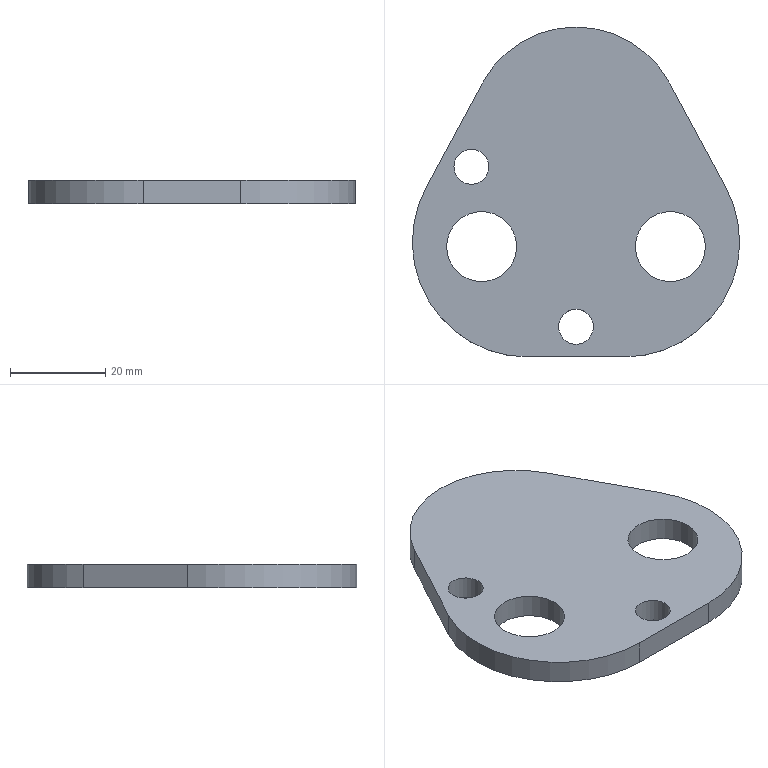Part | STEP file | 1_id374_x_t | 1 solid | 12 faces | box 68.793 x 69.35 x 5 mm | volume 16032 mm3 | cylinder 7 | plane 5 | commonest cylinder face diameters 7.35 x2 14.741 x2 48.276 x2 44.704 x1
STEP:
#1=CARTESIAN_POINT('',(0.,0.,0.));
#2=DIRECTION('',(0.,0.,1.));
#3=DIRECTION('',(1.,0.,0.));
#4=AXIS2_PLACEMENT_3D('',#1,#2,#3);
#5=CARTESIAN_POINT('',(924.47,166.067,104.675));
#6=VERTEX_POINT('',#5);
#7=CARTESIAN_POINT('',(903.208,130.502,104.675));
#8=VERTEX_POINT('',#7);
#9=CARTESIAN_POINT('',(903.208,154.64,104.675));
#10=DIRECTION('',(0.,0.,-1.));
#11=DIRECTION('',(1.,0.,0.));
#12=AXIS2_PLACEMENT_3D('',#9,#10,#11);
#13=CIRCLE('',#12,24.138);
#14=CARTESIAN_POINT('',(903.208,154.64,109.675));
#15=DIRECTION('',(0.,0.,-1.));
#16=DIRECTION('',(1.,0.,0.));
#17=AXIS2_PLACEMENT_3D('',#14,#15,#16);
#18=CYLINDRICAL_SURFACE('',#17,24.138);
#19=CARTESIAN_POINT('',(-6.283,5.));
#20=DIRECTION('',(1.,0.));
#21=VECTOR('',#20,1.);
#22=LINE('',#19,#21);
#23=(GEOMETRIC_REPRESENTATION_CONTEXT(2)PARAMETRIC_REPRESENTATION_CONTEXT()REPRESENTATION_CONTEXT('',''));
#24=DEFINITIONAL_REPRESENTATION('',(#22),#23);
#25=PCURVE('',#18,#24);
#26=CARTESIAN_POINT('',(892.95,177.5,104.675));
#27=DIRECTION('',(0.,0.,1.));
#28=DIRECTION('',(0.,1.,0.));
#29=AXIS2_PLACEMENT_3D('',#26,#27,#28);
#30=PLANE('',#29);
#31=CARTESIAN_POINT('',(-22.86,-34.396));
#32=CARTESIAN_POINT('',(-64.668,-34.396));
#33=CARTESIAN_POINT('',(-43.764,1.811));
#34=CARTESIAN_POINT('',(-22.86,38.018));
#35=CARTESIAN_POINT('',(-1.956,1.811));
#36=CARTESIAN_POINT('',(18.948,-34.396));
#37=CARTESIAN_POINT('',(-22.86,-34.396));
#38=(BOUNDED_CURVE()B_SPLINE_CURVE(2,(#31,#32,#33,#34,#35,#36,#37),.UNSPECIFIED.,.T.,.F.)B_SPLINE_CURVE_WITH_KNOTS((1,2,2,2,2,1),(-2.094,0.,2.094,4.189,6.283,8.378),.UNSPECIFIED.)CURVE()GEOMETRIC_REPRESENTATION_ITEM()RATIONAL_B_SPLINE_CURVE((1.,0.5,1.,0.5,1.,0.5,1.))REPRESENTATION_ITEM(''));
#39=(GEOMETRIC_REPRESENTATION_CONTEXT(2)PARAMETRIC_REPRESENTATION_CONTEXT()REPRESENTATION_CONTEXT('',''));
#40=DEFINITIONAL_REPRESENTATION('',(#38),#39);
#41=PCURVE('',#30,#40);
#42=SURFACE_CURVE('',#13,(#25,#41),.PCURVE_S1.);
#43=EDGE_CURVE('',#6,#8,#42,.T.);
#44=ORIENTED_EDGE('',*,*,#43,.F.);
#45=CARTESIAN_POINT('',(924.47,166.067,109.675));
#46=VERTEX_POINT('',#45);
#47=CARTESIAN_POINT('',(924.47,166.067,104.675));
#48=DIRECTION('',(0.,0.,1.));
#49=VECTOR('',#48,1.);
#50=LINE('',#47,#49);
#51=CARTESIAN_POINT('',(-0.4932,5.));
#52=DIRECTION('',(0.,-1.));
#53=VECTOR('',#52,1.);
#54=LINE('',#51,#53);
#55=(GEOMETRIC_REPRESENTATION_CONTEXT(2)PARAMETRIC_REPRESENTATION_CONTEXT()REPRESENTATION_CONTEXT('',''));
#56=DEFINITIONAL_REPRESENTATION('',(#54),#55);
#57=PCURVE('',#18,#56);
#58=CARTESIAN_POINT('',(924.304,166.376,109.675));
#59=DIRECTION('',(-0.8808,-0.4734,0.));
#60=DIRECTION('',(-0.4734,0.8808,0.));
#61=AXIS2_PLACEMENT_3D('',#58,#59,#60);
#62=PLANE('',#61);
#63=CARTESIAN_POINT('',(-0.3512,5.));
#64=DIRECTION('',(0.,-1.));
#65=VECTOR('',#64,1.);
#66=LINE('',#63,#65);
#67=(GEOMETRIC_REPRESENTATION_CONTEXT(2)PARAMETRIC_REPRESENTATION_CONTEXT()REPRESENTATION_CONTEXT('',''));
#68=DEFINITIONAL_REPRESENTATION('',(#66),#67);
#69=PCURVE('',#62,#68);
#70=SURFACE_CURVE('',#50,(#57,#69),.PCURVE_S1.);
#71=EDGE_CURVE('',#6,#46,#70,.T.);
#72=ORIENTED_EDGE('',*,*,#71,.T.);
#73=CARTESIAN_POINT('',(903.208,130.502,109.675));
#74=VERTEX_POINT('',#73);
#75=CARTESIAN_POINT('',(903.208,154.64,109.675));
#76=DIRECTION('',(0.,0.,1.));
#77=DIRECTION('',(0.,-1.,0.));
#78=AXIS2_PLACEMENT_3D('',#75,#76,#77);
#79=CIRCLE('',#78,24.138);
#80=CARTESIAN_POINT('',(1.571,0.));
#81=DIRECTION('',(-1.,0.));
#82=VECTOR('',#81,1.);
#83=LINE('',#80,#82);
#84=(GEOMETRIC_REPRESENTATION_CONTEXT(2)PARAMETRIC_REPRESENTATION_CONTEXT()REPRESENTATION_CONTEXT('',''));
#85=DEFINITIONAL_REPRESENTATION('',(#83),#84);
#86=PCURVE('',#18,#85);
#87=CARTESIAN_POINT('',(892.95,177.5,109.675));
#88=DIRECTION('',(0.,0.,1.));
#89=DIRECTION('',(0.,1.,0.));
#90=AXIS2_PLACEMENT_3D('',#87,#88,#89);
#91=PLANE('',#90);
#92=CARTESIAN_POINT('',(-22.86,-10.258));
#93=DIRECTION('',(-1.,0.));
#94=AXIS2_PLACEMENT_2D('',#92,#93);
#95=CIRCLE('',#94,24.138);
#96=(GEOMETRIC_REPRESENTATION_CONTEXT(2)PARAMETRIC_REPRESENTATION_CONTEXT()REPRESENTATION_CONTEXT('',''));
#97=DEFINITIONAL_REPRESENTATION('',(#95),#96);
#98=PCURVE('',#91,#97);
#99=SURFACE_CURVE('',#79,(#86,#98),.PCURVE_S1.);
#100=EDGE_CURVE('',#74,#46,#99,.T.);
#101=ORIENTED_EDGE('',*,*,#100,.F.);
#102=CARTESIAN_POINT('',(903.208,130.502,109.675));
#103=DIRECTION('',(0.,0.,-1.));
#104=VECTOR('',#103,1.);
#105=LINE('',#102,#104);
#106=CARTESIAN_POINT('',(1.571,0.));
#107=DIRECTION('',(0.,1.));
#108=VECTOR('',#107,1.);
#109=LINE('',#106,#108);
#110=(GEOMETRIC_REPRESENTATION_CONTEXT(2)PARAMETRIC_REPRESENTATION_CONTEXT()REPRESENTATION_CONTEXT('',''));
#111=DEFINITIONAL_REPRESENTATION('',(#109),#110);
#112=PCURVE('',#18,#111);
#113=CARTESIAN_POINT('',(883.044,130.502,109.675));
#114=DIRECTION('',(0.,1.,0.));
#115=DIRECTION('',(0.,0.,-1.));
#116=AXIS2_PLACEMENT_3D('',#113,#114,#115);
#117=PLANE('',#116);
#118=CARTESIAN_POINT('',(0.,-20.164));
#119=DIRECTION('',(1.,0.));
#120=VECTOR('',#119,1.);
#121=LINE('',#118,#120);
#122=(GEOMETRIC_REPRESENTATION_CONTEXT(2)PARAMETRIC_REPRESENTATION_CONTEXT()REPRESENTATION_CONTEXT('',''));
#123=DEFINITIONAL_REPRESENTATION('',(#121),#122);
#124=PCURVE('',#117,#123);
#125=SURFACE_CURVE('',#105,(#112,#124),.PCURVE_S1.);
#126=EDGE_CURVE('',#74,#8,#125,.T.);
#127=ORIENTED_EDGE('',*,*,#126,.T.);
#128=EDGE_LOOP('',(#44,#72,#101,#127));
#129=FACE_BOUND('',#128,.T.);
#130=ADVANCED_FACE('',(#129),#18,.T.);
#131=CARTESIAN_POINT('',(882.692,130.502,104.675));
#132=VERTEX_POINT('',#131);
#133=CARTESIAN_POINT('',(903.208,130.502,104.675));
#134=DIRECTION('',(-1.,0.,0.));
#135=VECTOR('',#134,1.);
#136=LINE('',#133,#135);
#137=CARTESIAN_POINT('',(-46.998,-10.258));
#138=DIRECTION('',(0.,1.));
#139=VECTOR('',#138,1.);
#140=LINE('',#137,#139);
#141=(GEOMETRIC_REPRESENTATION_CONTEXT(2)PARAMETRIC_REPRESENTATION_CONTEXT()REPRESENTATION_CONTEXT('',''));
#142=DEFINITIONAL_REPRESENTATION('',(#140),#141);
#143=PCURVE('',#30,#142);
#144=CARTESIAN_POINT('',(5.,-20.164));
#145=DIRECTION('',(0.,1.));
#146=VECTOR('',#145,1.);
#147=LINE('',#144,#146);
#148=(GEOMETRIC_REPRESENTATION_CONTEXT(2)PARAMETRIC_REPRESENTATION_CONTEXT()REPRESENTATION_CONTEXT('',''));
#149=DEFINITIONAL_REPRESENTATION('',(#147),#148);
#150=PCURVE('',#117,#149);
#151=SURFACE_CURVE('',#136,(#143,#150),.PCURVE_S1.);
#152=EDGE_CURVE('',#8,#132,#151,.T.);
#153=ORIENTED_EDGE('',*,*,#152,.T.);
#154=CARTESIAN_POINT('',(861.43,166.067,104.675));
#155=VERTEX_POINT('',#154);
#156=CARTESIAN_POINT('',(882.692,154.64,104.675));
#157=DIRECTION('',(0.,0.,-1.));
#158=DIRECTION('',(-1.,0.,0.));
#159=AXIS2_PLACEMENT_3D('',#156,#157,#158);
#160=CIRCLE('',#159,24.138);
#161=CARTESIAN_POINT('',(-22.86,34.396));
#162=CARTESIAN_POINT('',(18.948,34.396));
#163=CARTESIAN_POINT('',(-1.956,-1.811));
#164=CARTESIAN_POINT('',(-22.86,-38.018));
#165=CARTESIAN_POINT('',(-43.764,-1.811));
#166=CARTESIAN_POINT('',(-64.668,34.396));
#167=CARTESIAN_POINT('',(-22.86,34.396));
#168=(BOUNDED_CURVE()B_SPLINE_CURVE(2,(#161,#162,#163,#164,#165,#166,#167),.UNSPECIFIED.,.T.,.F.)B_SPLINE_CURVE_WITH_KNOTS((1,2,2,2,2,1),(-2.094,0.,2.094,4.189,6.283,8.378),.UNSPECIFIED.)CURVE()GEOMETRIC_REPRESENTATION_ITEM()RATIONAL_B_SPLINE_CURVE((1.,0.5,1.,0.5,1.,0.5,1.))REPRESENTATION_ITEM(''));
#169=(GEOMETRIC_REPRESENTATION_CONTEXT(2)PARAMETRIC_REPRESENTATION_CONTEXT()REPRESENTATION_CONTEXT('',''));
#170=DEFINITIONAL_REPRESENTATION('',(#168),#169);
#171=PCURVE('',#30,#170);
#172=CARTESIAN_POINT('',(882.692,154.64,109.675));
#173=DIRECTION('',(0.,0.,-1.));
#174=DIRECTION('',(1.,0.,0.));
#175=AXIS2_PLACEMENT_3D('',#172,#173,#174);
#176=CYLINDRICAL_SURFACE('',#175,24.138);
#177=CARTESIAN_POINT('',(-3.142,5.));
#178=DIRECTION('',(1.,0.));
#179=VECTOR('',#178,1.);
#180=LINE('',#177,#179);
#181=(GEOMETRIC_REPRESENTATION_CONTEXT(2)PARAMETRIC_REPRESENTATION_CONTEXT()REPRESENTATION_CONTEXT('',''));
#182=DEFINITIONAL_REPRESENTATION('',(#180),#181);
#183=PCURVE('',#176,#182);
#184=SURFACE_CURVE('',#160,(#171,#183),.PCURVE_S1.);
#185=EDGE_CURVE('',#132,#155,#184,.T.);
#186=ORIENTED_EDGE('',*,*,#185,.T.);
#187=CARTESIAN_POINT('',(873.261,188.082,104.675));
#188=VERTEX_POINT('',#187);
#189=CARTESIAN_POINT('',(861.43,166.067,104.675));
#190=DIRECTION('',(0.4734,0.8808,0.));
#191=VECTOR('',#190,1.);
#192=LINE('',#189,#191);
#193=CARTESIAN_POINT('',(-11.433,31.52));
#194=DIRECTION('',(0.8808,-0.4734));
#195=VECTOR('',#194,1.);
#196=LINE('',#193,#195);
#197=(GEOMETRIC_REPRESENTATION_CONTEXT(2)PARAMETRIC_REPRESENTATION_CONTEXT()REPRESENTATION_CONTEXT('',''));
#198=DEFINITIONAL_REPRESENTATION('',(#196),#197);
#199=PCURVE('',#30,#198);
#200=CARTESIAN_POINT('',(873.34,188.229,109.675));
#201=DIRECTION('',(0.8808,-0.4734,0.));
#202=DIRECTION('',(-0.4734,-0.8808,0.));
#203=AXIS2_PLACEMENT_3D('',#200,#201,#202);
#204=PLANE('',#203);
#205=CARTESIAN_POINT('',(25.159,5.));
#206=DIRECTION('',(-1.,0.));
#207=VECTOR('',#206,1.);
#208=LINE('',#205,#207);
#209=(GEOMETRIC_REPRESENTATION_CONTEXT(2)PARAMETRIC_REPRESENTATION_CONTEXT()REPRESENTATION_CONTEXT('',''));
#210=DEFINITIONAL_REPRESENTATION('',(#208),#209);
#211=PCURVE('',#204,#210);
#212=SURFACE_CURVE('',#192,(#199,#211),.PCURVE_S1.);
#213=EDGE_CURVE('',#155,#188,#212,.T.);
#214=ORIENTED_EDGE('',*,*,#213,.T.);
#215=CARTESIAN_POINT('',(912.639,188.082,104.675));
#216=VERTEX_POINT('',#215);
#217=CARTESIAN_POINT('',(892.95,177.5,104.675));
#218=DIRECTION('',(0.,0.,-1.));
#219=DIRECTION('',(-0.8808,0.4734,0.));
#220=AXIS2_PLACEMENT_3D('',#217,#218,#219);
#221=CIRCLE('',#220,22.352);
#222=CARTESIAN_POINT('',(10.582,19.689));
#223=CARTESIAN_POINT('',(44.683,1.361));
#224=CARTESIAN_POINT('',(11.76,-19.008));
#225=CARTESIAN_POINT('',(-21.163,-39.377));
#226=CARTESIAN_POINT('',(-22.342,-0.6804));
#227=CARTESIAN_POINT('',(-23.52,38.016));
#228=CARTESIAN_POINT('',(10.582,19.689));
#229=(BOUNDED_CURVE()B_SPLINE_CURVE(2,(#222,#223,#224,#225,#226,#227,#228),.UNSPECIFIED.,.T.,.F.)B_SPLINE_CURVE_WITH_KNOTS((1,2,2,2,2,1),(-2.094,0.,2.094,4.189,6.283,8.378),.UNSPECIFIED.)CURVE()GEOMETRIC_REPRESENTATION_ITEM()RATIONAL_B_SPLINE_CURVE((1.,0.5,1.,0.5,1.,0.5,1.))REPRESENTATION_ITEM(''));
#230=(GEOMETRIC_REPRESENTATION_CONTEXT(2)PARAMETRIC_REPRESENTATION_CONTEXT()REPRESENTATION_CONTEXT('',''));
#231=DEFINITIONAL_REPRESENTATION('',(#229),#230);
#232=PCURVE('',#30,#231);
#233=CARTESIAN_POINT('',(892.95,177.5,109.675));
#234=DIRECTION('',(0.,0.,-1.));
#235=DIRECTION('',(1.,0.,0.));
#236=AXIS2_PLACEMENT_3D('',#233,#234,#235);
#237=CYLINDRICAL_SURFACE('',#236,22.352);
#238=CARTESIAN_POINT('',(3.635,5.));
#239=DIRECTION('',(1.,0.));
#240=VECTOR('',#239,1.);
#241=LINE('',#238,#240);
#242=(GEOMETRIC_REPRESENTATION_CONTEXT(2)PARAMETRIC_REPRESENTATION_CONTEXT()REPRESENTATION_CONTEXT('',''));
#243=DEFINITIONAL_REPRESENTATION('',(#241),#242);
#244=PCURVE('',#237,#243);
#245=SURFACE_CURVE('',#221,(#232,#244),.PCURVE_S1.);
#246=EDGE_CURVE('',#188,#216,#245,.T.);
#247=ORIENTED_EDGE('',*,*,#246,.T.);
#248=CARTESIAN_POINT('',(912.639,188.082,104.675));
#249=DIRECTION('',(0.4734,-0.8808,0.));
#250=VECTOR('',#249,1.);
#251=LINE('',#248,#250);
#252=CARTESIAN_POINT('',(10.582,-19.689));
#253=DIRECTION('',(-0.8808,-0.4734));
#254=VECTOR('',#253,1.);
#255=LINE('',#252,#254);
#256=(GEOMETRIC_REPRESENTATION_CONTEXT(2)PARAMETRIC_REPRESENTATION_CONTEXT()REPRESENTATION_CONTEXT('',''));
#257=DEFINITIONAL_REPRESENTATION('',(#255),#256);
#258=PCURVE('',#30,#257);
#259=CARTESIAN_POINT('',(24.641,5.));
#260=DIRECTION('',(-1.,0.));
#261=VECTOR('',#260,1.);
#262=LINE('',#259,#261);
#263=(GEOMETRIC_REPRESENTATION_CONTEXT(2)PARAMETRIC_REPRESENTATION_CONTEXT()REPRESENTATION_CONTEXT('',''));
#264=DEFINITIONAL_REPRESENTATION('',(#262),#263);
#265=PCURVE('',#62,#264);
#266=SURFACE_CURVE('',#251,(#258,#265),.PCURVE_S1.);
#267=EDGE_CURVE('',#216,#6,#266,.T.);
#268=ORIENTED_EDGE('',*,*,#267,.T.);
#269=ORIENTED_EDGE('',*,*,#43,.T.);
#270=EDGE_LOOP('',(#153,#186,#214,#247,#268,#269));
#271=FACE_BOUND('',#270,.T.);
#272=CARTESIAN_POINT('',(874.629,170.49,104.675));
#273=VERTEX_POINT('',#272);
#274=CARTESIAN_POINT('',(870.954,170.49,104.675));
#275=DIRECTION('',(0.,0.,1.));
#276=DIRECTION('',(1.,0.,0.));
#277=AXIS2_PLACEMENT_3D('',#274,#275,#276);
#278=CIRCLE('',#277,3.675);
#279=CARTESIAN_POINT('',(-7.01,21.996));
#280=DIRECTION('',(0.,-1.));
#281=AXIS2_PLACEMENT_2D('',#279,#280);
#282=CIRCLE('',#281,3.675);
#283=(GEOMETRIC_REPRESENTATION_CONTEXT(2)PARAMETRIC_REPRESENTATION_CONTEXT()REPRESENTATION_CONTEXT('',''));
#284=DEFINITIONAL_REPRESENTATION('',(#282),#283);
#285=PCURVE('',#30,#284);
#286=CARTESIAN_POINT('',(870.954,170.49,109.675));
#287=DIRECTION('',(0.,0.,-1.));
#288=DIRECTION('',(1.,0.,0.));
#289=AXIS2_PLACEMENT_3D('',#286,#287,#288);
#290=CYLINDRICAL_SURFACE('',#289,3.675);
#291=CARTESIAN_POINT('',(6.283,5.));
#292=DIRECTION('',(-1.,0.));
#293=VECTOR('',#292,1.);
#294=LINE('',#291,#293);
#295=(GEOMETRIC_REPRESENTATION_CONTEXT(2)PARAMETRIC_REPRESENTATION_CONTEXT()REPRESENTATION_CONTEXT('',''));
#296=DEFINITIONAL_REPRESENTATION('',(#294),#295);
#297=PCURVE('',#290,#296);
#298=SURFACE_CURVE('',#278,(#285,#297),.PCURVE_S1.);
#299=EDGE_CURVE('',#273,#273,#298,.T.);
#300=ORIENTED_EDGE('',*,*,#299,.T.);
#301=EDGE_LOOP('',(#300));
#302=FACE_BOUND('',#301,.T.);
#303=CARTESIAN_POINT('',(920.158,153.675,104.675));
#304=VERTEX_POINT('',#303);
#305=CARTESIAN_POINT('',(912.787,153.675,104.675));
#306=DIRECTION('',(0.,0.,1.));
#307=DIRECTION('',(1.,0.,0.));
#308=AXIS2_PLACEMENT_3D('',#305,#306,#307);
#309=CIRCLE('',#308,7.371);
#310=CARTESIAN_POINT('',(-23.825,-19.837));
#311=DIRECTION('',(0.,-1.));
#312=AXIS2_PLACEMENT_2D('',#310,#311);
#313=CIRCLE('',#312,7.371);
#314=(GEOMETRIC_REPRESENTATION_CONTEXT(2)PARAMETRIC_REPRESENTATION_CONTEXT()REPRESENTATION_CONTEXT('',''));
#315=DEFINITIONAL_REPRESENTATION('',(#313),#314);
#316=PCURVE('',#30,#315);
#317=CARTESIAN_POINT('',(912.787,153.675,109.675));
#318=DIRECTION('',(0.,0.,-1.));
#319=DIRECTION('',(1.,0.,0.));
#320=AXIS2_PLACEMENT_3D('',#317,#318,#319);
#321=CYLINDRICAL_SURFACE('',#320,7.371);
#322=CARTESIAN_POINT('',(6.283,5.));
#323=DIRECTION('',(-1.,0.));
#324=VECTOR('',#323,1.);
#325=LINE('',#322,#324);
#326=(GEOMETRIC_REPRESENTATION_CONTEXT(2)PARAMETRIC_REPRESENTATION_CONTEXT()REPRESENTATION_CONTEXT('',''));
#327=DEFINITIONAL_REPRESENTATION('',(#325),#326);
#328=PCURVE('',#321,#327);
#329=SURFACE_CURVE('',#309,(#316,#328),.PCURVE_S1.);
#330=EDGE_CURVE('',#304,#304,#329,.T.);
#331=ORIENTED_EDGE('',*,*,#330,.T.);
#332=EDGE_LOOP('',(#331));
#333=FACE_BOUND('',#332,.T.);
#334=CARTESIAN_POINT('',(880.483,153.675,104.675));
#335=VERTEX_POINT('',#334);
#336=CARTESIAN_POINT('',(873.113,153.675,104.675));
#337=DIRECTION('',(0.,0.,1.));
#338=DIRECTION('',(1.,0.,0.));
#339=AXIS2_PLACEMENT_3D('',#336,#337,#338);
#340=CIRCLE('',#339,7.371);
#341=CARTESIAN_POINT('',(-23.825,19.837));
#342=DIRECTION('',(0.,-1.));
#343=AXIS2_PLACEMENT_2D('',#341,#342);
#344=CIRCLE('',#343,7.371);
#345=(GEOMETRIC_REPRESENTATION_CONTEXT(2)PARAMETRIC_REPRESENTATION_CONTEXT()REPRESENTATION_CONTEXT('',''));
#346=DEFINITIONAL_REPRESENTATION('',(#344),#345);
#347=PCURVE('',#30,#346);
#348=CARTESIAN_POINT('',(873.113,153.675,109.675));
#349=DIRECTION('',(0.,0.,-1.));
#350=DIRECTION('',(1.,0.,0.));
#351=AXIS2_PLACEMENT_3D('',#348,#349,#350);
#352=CYLINDRICAL_SURFACE('',#351,7.371);
#353=CARTESIAN_POINT('',(6.283,5.));
#354=DIRECTION('',(-1.,0.));
#355=VECTOR('',#354,1.);
#356=LINE('',#353,#355);
#357=(GEOMETRIC_REPRESENTATION_CONTEXT(2)PARAMETRIC_REPRESENTATION_CONTEXT()REPRESENTATION_CONTEXT('',''));
#358=DEFINITIONAL_REPRESENTATION('',(#356),#357);
#359=PCURVE('',#352,#358);
#360=SURFACE_CURVE('',#340,(#347,#359),.PCURVE_S1.);
#361=EDGE_CURVE('',#335,#335,#360,.T.);
#362=ORIENTED_EDGE('',*,*,#361,.T.);
#363=EDGE_LOOP('',(#362));
#364=FACE_BOUND('',#363,.T.);
#365=CARTESIAN_POINT('',(896.625,136.86,104.675));
#366=VERTEX_POINT('',#365);
#367=CARTESIAN_POINT('',(892.95,136.86,104.675));
#368=DIRECTION('',(0.,0.,1.));
#369=DIRECTION('',(1.,0.,0.));
#370=AXIS2_PLACEMENT_3D('',#367,#368,#369);
#371=CIRCLE('',#370,3.675);
#372=CARTESIAN_POINT('',(-40.64,0.));
#373=DIRECTION('',(0.,-1.));
#374=AXIS2_PLACEMENT_2D('',#372,#373);
#375=CIRCLE('',#374,3.675);
#376=(GEOMETRIC_REPRESENTATION_CONTEXT(2)PARAMETRIC_REPRESENTATION_CONTEXT()REPRESENTATION_CONTEXT('',''));
#377=DEFINITIONAL_REPRESENTATION('',(#375),#376);
#378=PCURVE('',#30,#377);
#379=CARTESIAN_POINT('',(892.95,136.86,109.675));
#380=DIRECTION('',(0.,0.,-1.));
#381=DIRECTION('',(1.,0.,0.));
#382=AXIS2_PLACEMENT_3D('',#379,#380,#381);
#383=CYLINDRICAL_SURFACE('',#382,3.675);
#384=CARTESIAN_POINT('',(6.283,5.));
#385=DIRECTION('',(-1.,0.));
#386=VECTOR('',#385,1.);
#387=LINE('',#384,#386);
#388=(GEOMETRIC_REPRESENTATION_CONTEXT(2)PARAMETRIC_REPRESENTATION_CONTEXT()REPRESENTATION_CONTEXT('',''));
#389=DEFINITIONAL_REPRESENTATION('',(#387),#388);
#390=PCURVE('',#383,#389);
#391=SURFACE_CURVE('',#371,(#378,#390),.PCURVE_S1.);
#392=EDGE_CURVE('',#366,#366,#391,.T.);
#393=ORIENTED_EDGE('',*,*,#392,.T.);
#394=EDGE_LOOP('',(#393));
#395=FACE_BOUND('',#394,.T.);
#396=ADVANCED_FACE('',(#271,#302,#333,#364,#395),#30,.F.);
#397=CARTESIAN_POINT('',(912.639,188.082,109.675));
#398=VERTEX_POINT('',#397);
#399=CARTESIAN_POINT('',(912.639,188.082,109.675));
#400=DIRECTION('',(0.,0.,-1.));
#401=VECTOR('',#400,1.);
#402=LINE('',#399,#401);
#403=CARTESIAN_POINT('',(24.641,0.));
#404=DIRECTION('',(0.,1.));
#405=VECTOR('',#404,1.);
#406=LINE('',#403,#405);
#407=(GEOMETRIC_REPRESENTATION_CONTEXT(2)PARAMETRIC_REPRESENTATION_CONTEXT()REPRESENTATION_CONTEXT('',''));
#408=DEFINITIONAL_REPRESENTATION('',(#406),#407);
#409=PCURVE('',#62,#408);
#410=CARTESIAN_POINT('',(5.79,0.));
#411=DIRECTION('',(0.,1.));
#412=VECTOR('',#411,1.);
#413=LINE('',#410,#412);
#414=(GEOMETRIC_REPRESENTATION_CONTEXT(2)PARAMETRIC_REPRESENTATION_CONTEXT()REPRESENTATION_CONTEXT('',''));
#415=DEFINITIONAL_REPRESENTATION('',(#413),#414);
#416=PCURVE('',#237,#415);
#417=SURFACE_CURVE('',#402,(#409,#416),.PCURVE_S1.);
#418=EDGE_CURVE('',#398,#216,#417,.T.);
#419=ORIENTED_EDGE('',*,*,#418,.F.);
#420=CARTESIAN_POINT('',(924.47,166.067,109.675));
#421=DIRECTION('',(-0.4734,0.8808,0.));
#422=VECTOR('',#421,1.);
#423=LINE('',#420,#422);
#424=CARTESIAN_POINT('',(-0.3512,0.));
#425=DIRECTION('',(1.,0.));
#426=VECTOR('',#425,1.);
#427=LINE('',#424,#426);
#428=(GEOMETRIC_REPRESENTATION_CONTEXT(2)PARAMETRIC_REPRESENTATION_CONTEXT()REPRESENTATION_CONTEXT('',''));
#429=DEFINITIONAL_REPRESENTATION('',(#427),#428);
#430=PCURVE('',#62,#429);
#431=CARTESIAN_POINT('',(-11.433,-31.52));
#432=DIRECTION('',(0.8808,0.4734));
#433=VECTOR('',#432,1.);
#434=LINE('',#431,#433);
#435=(GEOMETRIC_REPRESENTATION_CONTEXT(2)PARAMETRIC_REPRESENTATION_CONTEXT()REPRESENTATION_CONTEXT('',''));
#436=DEFINITIONAL_REPRESENTATION('',(#434),#435);
#437=PCURVE('',#91,#436);
#438=SURFACE_CURVE('',#423,(#430,#437),.PCURVE_S1.);
#439=EDGE_CURVE('',#46,#398,#438,.T.);
#440=ORIENTED_EDGE('',*,*,#439,.F.);
#441=ORIENTED_EDGE('',*,*,#71,.F.);
#442=ORIENTED_EDGE('',*,*,#267,.F.);
#443=EDGE_LOOP('',(#419,#440,#441,#442));
#444=FACE_BOUND('',#443,.T.);
#445=ADVANCED_FACE('',(#444),#62,.F.);
#446=ORIENTED_EDGE('',*,*,#439,.T.);
#447=CARTESIAN_POINT('',(873.261,188.082,109.675));
#448=VERTEX_POINT('',#447);
#449=CARTESIAN_POINT('',(892.95,177.5,109.675));
#450=DIRECTION('',(0.,0.,1.));
#451=DIRECTION('',(0.8808,0.4734,0.));
#452=AXIS2_PLACEMENT_3D('',#449,#450,#451);
#453=CIRCLE('',#452,22.352);
#454=CARTESIAN_POINT('',(0.,0.));
#455=DIRECTION('',(0.4734,-0.8808));
#456=AXIS2_PLACEMENT_2D('',#454,#455);
#457=CIRCLE('',#456,22.352);
#458=(GEOMETRIC_REPRESENTATION_CONTEXT(2)PARAMETRIC_REPRESENTATION_CONTEXT()REPRESENTATION_CONTEXT('',''));
#459=DEFINITIONAL_REPRESENTATION('',(#457),#458);
#460=PCURVE('',#91,#459);
#461=CARTESIAN_POINT('',(12.073,0.));
#462=DIRECTION('',(-1.,0.));
#463=VECTOR('',#462,1.);
#464=LINE('',#461,#463);
#465=(GEOMETRIC_REPRESENTATION_CONTEXT(2)PARAMETRIC_REPRESENTATION_CONTEXT()REPRESENTATION_CONTEXT('',''));
#466=DEFINITIONAL_REPRESENTATION('',(#464),#465);
#467=PCURVE('',#237,#466);
#468=SURFACE_CURVE('',#453,(#460,#467),.PCURVE_S1.);
#469=EDGE_CURVE('',#398,#448,#468,.T.);
#470=ORIENTED_EDGE('',*,*,#469,.T.);
#471=CARTESIAN_POINT('',(861.43,166.067,109.675));
#472=VERTEX_POINT('',#471);
#473=CARTESIAN_POINT('',(873.261,188.082,109.675));
#474=DIRECTION('',(-0.4734,-0.8808,0.));
#475=VECTOR('',#474,1.);
#476=LINE('',#473,#475);
#477=CARTESIAN_POINT('',(10.582,19.689));
#478=DIRECTION('',(-0.8808,0.4734));
#479=VECTOR('',#478,1.);
#480=LINE('',#477,#479);
#481=(GEOMETRIC_REPRESENTATION_CONTEXT(2)PARAMETRIC_REPRESENTATION_CONTEXT()REPRESENTATION_CONTEXT('',''));
#482=DEFINITIONAL_REPRESENTATION('',(#480),#481);
#483=PCURVE('',#91,#482);
#484=CARTESIAN_POINT('',(0.1669,0.));
#485=DIRECTION('',(1.,0.));
#486=VECTOR('',#485,1.);
#487=LINE('',#484,#486);
#488=(GEOMETRIC_REPRESENTATION_CONTEXT(2)PARAMETRIC_REPRESENTATION_CONTEXT()REPRESENTATION_CONTEXT('',''));
#489=DEFINITIONAL_REPRESENTATION('',(#487),#488);
#490=PCURVE('',#204,#489);
#491=SURFACE_CURVE('',#476,(#483,#490),.PCURVE_S1.);
#492=EDGE_CURVE('',#448,#472,#491,.T.);
#493=ORIENTED_EDGE('',*,*,#492,.T.);
#494=CARTESIAN_POINT('',(882.692,130.502,109.675));
#495=VERTEX_POINT('',#494);
#496=CARTESIAN_POINT('',(882.692,154.64,109.675));
#497=DIRECTION('',(0.,0.,1.));
#498=DIRECTION('',(-1.,0.,0.));
#499=AXIS2_PLACEMENT_3D('',#496,#497,#498);
#500=CIRCLE('',#499,24.138);
#501=CARTESIAN_POINT('',(-22.86,10.258));
#502=DIRECTION('',(0.,1.));
#503=AXIS2_PLACEMENT_2D('',#501,#502);
#504=CIRCLE('',#503,24.138);
#505=(GEOMETRIC_REPRESENTATION_CONTEXT(2)PARAMETRIC_REPRESENTATION_CONTEXT()REPRESENTATION_CONTEXT('',''));
#506=DEFINITIONAL_REPRESENTATION('',(#504),#505);
#507=PCURVE('',#91,#506);
#508=CARTESIAN_POINT('',(9.425,0.));
#509=DIRECTION('',(-1.,0.));
#510=VECTOR('',#509,1.);
#511=LINE('',#508,#510);
#512=(GEOMETRIC_REPRESENTATION_CONTEXT(2)PARAMETRIC_REPRESENTATION_CONTEXT()REPRESENTATION_CONTEXT('',''));
#513=DEFINITIONAL_REPRESENTATION('',(#511),#512);
#514=PCURVE('',#176,#513);
#515=SURFACE_CURVE('',#500,(#507,#514),.PCURVE_S1.);
#516=EDGE_CURVE('',#472,#495,#515,.T.);
#517=ORIENTED_EDGE('',*,*,#516,.T.);
#518=CARTESIAN_POINT('',(903.208,130.502,109.675));
#519=DIRECTION('',(-1.,0.,0.));
#520=VECTOR('',#519,1.);
#521=LINE('',#518,#520);
#522=CARTESIAN_POINT('',(-46.998,-10.258));
#523=DIRECTION('',(0.,1.));
#524=VECTOR('',#523,1.);
#525=LINE('',#522,#524);
#526=(GEOMETRIC_REPRESENTATION_CONTEXT(2)PARAMETRIC_REPRESENTATION_CONTEXT()REPRESENTATION_CONTEXT('',''));
#527=DEFINITIONAL_REPRESENTATION('',(#525),#526);
#528=PCURVE('',#91,#527);
#529=CARTESIAN_POINT('',(0.,-20.164));
#530=DIRECTION('',(0.,1.));
#531=VECTOR('',#530,1.);
#532=LINE('',#529,#531);
#533=(GEOMETRIC_REPRESENTATION_CONTEXT(2)PARAMETRIC_REPRESENTATION_CONTEXT()REPRESENTATION_CONTEXT('',''));
#534=DEFINITIONAL_REPRESENTATION('',(#532),#533);
#535=PCURVE('',#117,#534);
#536=SURFACE_CURVE('',#521,(#528,#535),.PCURVE_S1.);
#537=EDGE_CURVE('',#74,#495,#536,.T.);
#538=ORIENTED_EDGE('',*,*,#537,.F.);
#539=ORIENTED_EDGE('',*,*,#100,.T.);
#540=EDGE_LOOP('',(#446,#470,#493,#517,#538,#539));
#541=FACE_BOUND('',#540,.T.);
#542=CARTESIAN_POINT('',(874.629,170.49,109.675));
#543=VERTEX_POINT('',#542);
#544=CARTESIAN_POINT('',(870.954,170.49,109.675));
#545=DIRECTION('',(0.,0.,-1.));
#546=DIRECTION('',(1.,0.,0.));
#547=AXIS2_PLACEMENT_3D('',#544,#545,#546);
#548=CIRCLE('',#547,3.675);
#549=CARTESIAN_POINT('',(-7.01,18.321));
#550=CARTESIAN_POINT('',(-13.376,18.321));
#551=CARTESIAN_POINT('',(-10.193,23.834));
#552=CARTESIAN_POINT('',(-7.01,29.346));
#553=CARTESIAN_POINT('',(-3.828,23.834));
#554=CARTESIAN_POINT('',(-0.6451,18.321));
#555=CARTESIAN_POINT('',(-7.01,18.321));
#556=(BOUNDED_CURVE()B_SPLINE_CURVE(2,(#549,#550,#551,#552,#553,#554,#555),.UNSPECIFIED.,.T.,.F.)B_SPLINE_CURVE_WITH_KNOTS((1,2,2,2,2,1),(-2.094,0.,2.094,4.189,6.283,8.378),.UNSPECIFIED.)CURVE()GEOMETRIC_REPRESENTATION_ITEM()RATIONAL_B_SPLINE_CURVE((1.,0.5,1.,0.5,1.,0.5,1.))REPRESENTATION_ITEM(''));
#557=(GEOMETRIC_REPRESENTATION_CONTEXT(2)PARAMETRIC_REPRESENTATION_CONTEXT()REPRESENTATION_CONTEXT('',''));
#558=DEFINITIONAL_REPRESENTATION('',(#556),#557);
#559=PCURVE('',#91,#558);
#560=CARTESIAN_POINT('',(0.,0.));
#561=DIRECTION('',(1.,0.));
#562=VECTOR('',#561,1.);
#563=LINE('',#560,#562);
#564=(GEOMETRIC_REPRESENTATION_CONTEXT(2)PARAMETRIC_REPRESENTATION_CONTEXT()REPRESENTATION_CONTEXT('',''));
#565=DEFINITIONAL_REPRESENTATION('',(#563),#564);
#566=PCURVE('',#290,#565);
#567=SURFACE_CURVE('',#548,(#559,#566),.PCURVE_S1.);
#568=EDGE_CURVE('',#543,#543,#567,.T.);
#569=ORIENTED_EDGE('',*,*,#568,.T.);
#570=EDGE_LOOP('',(#569));
#571=FACE_BOUND('',#570,.T.);
#572=CARTESIAN_POINT('',(920.158,153.675,109.675));
#573=VERTEX_POINT('',#572);
#574=CARTESIAN_POINT('',(912.787,153.675,109.675));
#575=DIRECTION('',(0.,0.,-1.));
#576=DIRECTION('',(1.,0.,0.));
#577=AXIS2_PLACEMENT_3D('',#574,#575,#576);
#578=CIRCLE('',#577,7.371);
#579=CARTESIAN_POINT('',(-23.825,-27.208));
#580=CARTESIAN_POINT('',(-36.592,-27.208));
#581=CARTESIAN_POINT('',(-30.208,-16.152));
#582=CARTESIAN_POINT('',(-23.825,-5.096));
#583=CARTESIAN_POINT('',(-17.442,-16.152));
#584=CARTESIAN_POINT('',(-11.059,-27.208));
#585=CARTESIAN_POINT('',(-23.825,-27.208));
#586=(BOUNDED_CURVE()B_SPLINE_CURVE(2,(#579,#580,#581,#582,#583,#584,#585),.UNSPECIFIED.,.T.,.F.)B_SPLINE_CURVE_WITH_KNOTS((1,2,2,2,2,1),(-2.094,0.,2.094,4.189,6.283,8.378),.UNSPECIFIED.)CURVE()GEOMETRIC_REPRESENTATION_ITEM()RATIONAL_B_SPLINE_CURVE((1.,0.5,1.,0.5,1.,0.5,1.))REPRESENTATION_ITEM(''));
#587=(GEOMETRIC_REPRESENTATION_CONTEXT(2)PARAMETRIC_REPRESENTATION_CONTEXT()REPRESENTATION_CONTEXT('',''));
#588=DEFINITIONAL_REPRESENTATION('',(#586),#587);
#589=PCURVE('',#91,#588);
#590=CARTESIAN_POINT('',(0.,0.));
#591=DIRECTION('',(1.,0.));
#592=VECTOR('',#591,1.);
#593=LINE('',#590,#592);
#594=(GEOMETRIC_REPRESENTATION_CONTEXT(2)PARAMETRIC_REPRESENTATION_CONTEXT()REPRESENTATION_CONTEXT('',''));
#595=DEFINITIONAL_REPRESENTATION('',(#593),#594);
#596=PCURVE('',#321,#595);
#597=SURFACE_CURVE('',#578,(#589,#596),.PCURVE_S1.);
#598=EDGE_CURVE('',#573,#573,#597,.T.);
#599=ORIENTED_EDGE('',*,*,#598,.T.);
#600=EDGE_LOOP('',(#599));
#601=FACE_BOUND('',#600,.T.);
#602=CARTESIAN_POINT('',(880.483,153.675,109.675));
#603=VERTEX_POINT('',#602);
#604=CARTESIAN_POINT('',(873.113,153.675,109.675));
#605=DIRECTION('',(0.,0.,-1.));
#606=DIRECTION('',(1.,0.,0.));
#607=AXIS2_PLACEMENT_3D('',#604,#605,#606);
#608=CIRCLE('',#607,7.371);
#609=CARTESIAN_POINT('',(-23.825,12.467));
#610=CARTESIAN_POINT('',(-36.592,12.467));
#611=CARTESIAN_POINT('',(-30.208,23.523));
#612=CARTESIAN_POINT('',(-23.825,34.579));
#613=CARTESIAN_POINT('',(-17.442,23.523));
#614=CARTESIAN_POINT('',(-11.059,12.467));
#615=CARTESIAN_POINT('',(-23.825,12.467));
#616=(BOUNDED_CURVE()B_SPLINE_CURVE(2,(#609,#610,#611,#612,#613,#614,#615),.UNSPECIFIED.,.T.,.F.)B_SPLINE_CURVE_WITH_KNOTS((1,2,2,2,2,1),(-2.094,0.,2.094,4.189,6.283,8.378),.UNSPECIFIED.)CURVE()GEOMETRIC_REPRESENTATION_ITEM()RATIONAL_B_SPLINE_CURVE((1.,0.5,1.,0.5,1.,0.5,1.))REPRESENTATION_ITEM(''));
#617=(GEOMETRIC_REPRESENTATION_CONTEXT(2)PARAMETRIC_REPRESENTATION_CONTEXT()REPRESENTATION_CONTEXT('',''));
#618=DEFINITIONAL_REPRESENTATION('',(#616),#617);
#619=PCURVE('',#91,#618);
#620=CARTESIAN_POINT('',(0.,0.));
#621=DIRECTION('',(1.,0.));
#622=VECTOR('',#621,1.);
#623=LINE('',#620,#622);
#624=(GEOMETRIC_REPRESENTATION_CONTEXT(2)PARAMETRIC_REPRESENTATION_CONTEXT()REPRESENTATION_CONTEXT('',''));
#625=DEFINITIONAL_REPRESENTATION('',(#623),#624);
#626=PCURVE('',#352,#625);
#627=SURFACE_CURVE('',#608,(#619,#626),.PCURVE_S1.);
#628=EDGE_CURVE('',#603,#603,#627,.T.);
#629=ORIENTED_EDGE('',*,*,#628,.T.);
#630=EDGE_LOOP('',(#629));
#631=FACE_BOUND('',#630,.T.);
#632=CARTESIAN_POINT('',(896.625,136.86,109.675));
#633=VERTEX_POINT('',#632);
#634=CARTESIAN_POINT('',(892.95,136.86,109.675));
#635=DIRECTION('',(0.,0.,-1.));
#636=DIRECTION('',(1.,0.,0.));
#637=AXIS2_PLACEMENT_3D('',#634,#635,#636);
#638=CIRCLE('',#637,3.675);
#639=CARTESIAN_POINT('',(-40.64,-3.675));
#640=CARTESIAN_POINT('',(-47.005,-3.675));
#641=CARTESIAN_POINT('',(-43.823,1.837));
#642=CARTESIAN_POINT('',(-40.64,7.35));
#643=CARTESIAN_POINT('',(-37.457,1.837));
#644=CARTESIAN_POINT('',(-34.275,-3.675));
#645=CARTESIAN_POINT('',(-40.64,-3.675));
#646=(BOUNDED_CURVE()B_SPLINE_CURVE(2,(#639,#640,#641,#642,#643,#644,#645),.UNSPECIFIED.,.T.,.F.)B_SPLINE_CURVE_WITH_KNOTS((1,2,2,2,2,1),(-2.094,0.,2.094,4.189,6.283,8.378),.UNSPECIFIED.)CURVE()GEOMETRIC_REPRESENTATION_ITEM()RATIONAL_B_SPLINE_CURVE((1.,0.5,1.,0.5,1.,0.5,1.))REPRESENTATION_ITEM(''));
#647=(GEOMETRIC_REPRESENTATION_CONTEXT(2)PARAMETRIC_REPRESENTATION_CONTEXT()REPRESENTATION_CONTEXT('',''));
#648=DEFINITIONAL_REPRESENTATION('',(#646),#647);
#649=PCURVE('',#91,#648);
#650=CARTESIAN_POINT('',(0.,0.));
#651=DIRECTION('',(1.,0.));
#652=VECTOR('',#651,1.);
#653=LINE('',#650,#652);
#654=(GEOMETRIC_REPRESENTATION_CONTEXT(2)PARAMETRIC_REPRESENTATION_CONTEXT()REPRESENTATION_CONTEXT('',''));
#655=DEFINITIONAL_REPRESENTATION('',(#653),#654);
#656=PCURVE('',#383,#655);
#657=SURFACE_CURVE('',#638,(#649,#656),.PCURVE_S1.);
#658=EDGE_CURVE('',#633,#633,#657,.T.);
#659=ORIENTED_EDGE('',*,*,#658,.T.);
#660=EDGE_LOOP('',(#659));
#661=FACE_BOUND('',#660,.T.);
#662=ADVANCED_FACE('',(#541,#571,#601,#631,#661),#91,.T.);
#663=ORIENTED_EDGE('',*,*,#126,.F.);
#664=ORIENTED_EDGE('',*,*,#537,.T.);
#665=CARTESIAN_POINT('',(882.692,130.502,104.675));
#666=DIRECTION('',(0.,0.,1.));
#667=VECTOR('',#666,1.);
#668=LINE('',#665,#667);
#669=CARTESIAN_POINT('',(5.,0.3524));
#670=DIRECTION('',(-1.,0.));
#671=VECTOR('',#670,1.);
#672=LINE('',#669,#671);
#673=(GEOMETRIC_REPRESENTATION_CONTEXT(2)PARAMETRIC_REPRESENTATION_CONTEXT()REPRESENTATION_CONTEXT('',''));
#674=DEFINITIONAL_REPRESENTATION('',(#672),#673);
#675=PCURVE('',#117,#674);
#676=CARTESIAN_POINT('',(1.571,5.));
#677=DIRECTION('',(0.,-1.));
#678=VECTOR('',#677,1.);
#679=LINE('',#676,#678);
#680=(GEOMETRIC_REPRESENTATION_CONTEXT(2)PARAMETRIC_REPRESENTATION_CONTEXT()REPRESENTATION_CONTEXT('',''));
#681=DEFINITIONAL_REPRESENTATION('',(#679),#680);
#682=PCURVE('',#176,#681);
#683=SURFACE_CURVE('',#668,(#675,#682),.PCURVE_S1.);
#684=EDGE_CURVE('',#132,#495,#683,.T.);
#685=ORIENTED_EDGE('',*,*,#684,.F.);
#686=ORIENTED_EDGE('',*,*,#152,.F.);
#687=EDGE_LOOP('',(#663,#664,#685,#686));
#688=FACE_BOUND('',#687,.T.);
#689=ADVANCED_FACE('',(#688),#117,.F.);
#690=ORIENTED_EDGE('',*,*,#185,.F.);
#691=ORIENTED_EDGE('',*,*,#684,.T.);
#692=ORIENTED_EDGE('',*,*,#516,.F.);
#693=CARTESIAN_POINT('',(861.43,166.067,109.675));
#694=DIRECTION('',(0.,0.,-1.));
#695=VECTOR('',#694,1.);
#696=LINE('',#693,#695);
#697=CARTESIAN_POINT('',(3.635,0.));
#698=DIRECTION('',(0.,1.));
#699=VECTOR('',#698,1.);
#700=LINE('',#697,#699);
#701=(GEOMETRIC_REPRESENTATION_CONTEXT(2)PARAMETRIC_REPRESENTATION_CONTEXT()REPRESENTATION_CONTEXT('',''));
#702=DEFINITIONAL_REPRESENTATION('',(#700),#701);
#703=PCURVE('',#176,#702);
#704=CARTESIAN_POINT('',(25.159,0.));
#705=DIRECTION('',(0.,1.));
#706=VECTOR('',#705,1.);
#707=LINE('',#704,#706);
#708=(GEOMETRIC_REPRESENTATION_CONTEXT(2)PARAMETRIC_REPRESENTATION_CONTEXT()REPRESENTATION_CONTEXT('',''));
#709=DEFINITIONAL_REPRESENTATION('',(#707),#708);
#710=PCURVE('',#204,#709);
#711=SURFACE_CURVE('',#696,(#703,#710),.PCURVE_S1.);
#712=EDGE_CURVE('',#472,#155,#711,.T.);
#713=ORIENTED_EDGE('',*,*,#712,.T.);
#714=EDGE_LOOP('',(#690,#691,#692,#713));
#715=FACE_BOUND('',#714,.T.);
#716=ADVANCED_FACE('',(#715),#176,.T.);
#717=ORIENTED_EDGE('',*,*,#712,.F.);
#718=ORIENTED_EDGE('',*,*,#492,.F.);
#719=CARTESIAN_POINT('',(873.261,188.082,104.675));
#720=DIRECTION('',(0.,0.,1.));
#721=VECTOR('',#720,1.);
#722=LINE('',#719,#721);
#723=CARTESIAN_POINT('',(0.1669,5.));
#724=DIRECTION('',(0.,-1.));
#725=VECTOR('',#724,1.);
#726=LINE('',#723,#725);
#727=(GEOMETRIC_REPRESENTATION_CONTEXT(2)PARAMETRIC_REPRESENTATION_CONTEXT()REPRESENTATION_CONTEXT('',''));
#728=DEFINITIONAL_REPRESENTATION('',(#726),#727);
#729=PCURVE('',#204,#728);
#730=CARTESIAN_POINT('',(3.635,5.));
#731=DIRECTION('',(0.,-1.));
#732=VECTOR('',#731,1.);
#733=LINE('',#730,#732);
#734=(GEOMETRIC_REPRESENTATION_CONTEXT(2)PARAMETRIC_REPRESENTATION_CONTEXT()REPRESENTATION_CONTEXT('',''));
#735=DEFINITIONAL_REPRESENTATION('',(#733),#734);
#736=PCURVE('',#237,#735);
#737=SURFACE_CURVE('',#722,(#729,#736),.PCURVE_S1.);
#738=EDGE_CURVE('',#188,#448,#737,.T.);
#739=ORIENTED_EDGE('',*,*,#738,.F.);
#740=ORIENTED_EDGE('',*,*,#213,.F.);
#741=EDGE_LOOP('',(#717,#718,#739,#740));
#742=FACE_BOUND('',#741,.T.);
#743=ADVANCED_FACE('',(#742),#204,.F.);
#744=ORIENTED_EDGE('',*,*,#738,.T.);
#745=ORIENTED_EDGE('',*,*,#469,.F.);
#746=ORIENTED_EDGE('',*,*,#418,.T.);
#747=ORIENTED_EDGE('',*,*,#246,.F.);
#748=EDGE_LOOP('',(#744,#745,#746,#747));
#749=FACE_BOUND('',#748,.T.);
#750=ADVANCED_FACE('',(#749),#237,.T.);
#751=ORIENTED_EDGE('',*,*,#299,.T.);
#752=CARTESIAN_POINT('',(874.629,170.49,109.675));
#753=CARTESIAN_POINT('',(874.629,170.49,104.675));
#754=B_SPLINE_CURVE_WITH_KNOTS('',1,(#752,#753),.UNSPECIFIED.,.F.,.F.,(2,2),(0.,5.),.PIECEWISE_BEZIER_KNOTS.);
#755=CARTESIAN_POINT('',(0.,0.));
#756=DIRECTION('',(0.,1.));
#757=VECTOR('',#756,1.);
#758=LINE('',#755,#757);
#759=(GEOMETRIC_REPRESENTATION_CONTEXT(2)PARAMETRIC_REPRESENTATION_CONTEXT()REPRESENTATION_CONTEXT('',''));
#760=DEFINITIONAL_REPRESENTATION('',(#758),#759);
#761=PCURVE('',#290,#760);
#762=CARTESIAN_POINT('',(6.283,0.));
#763=DIRECTION('',(0.,1.));
#764=VECTOR('',#763,1.);
#765=LINE('',#762,#764);
#766=(GEOMETRIC_REPRESENTATION_CONTEXT(2)PARAMETRIC_REPRESENTATION_CONTEXT()REPRESENTATION_CONTEXT('',''));
#767=DEFINITIONAL_REPRESENTATION('',(#765),#766);
#768=PCURVE('',#290,#767);
#769=SEAM_CURVE('',#754,(#761,#768),.PCURVE_S1.);
#770=EDGE_CURVE('',#543,#273,#769,.T.);
#771=ORIENTED_EDGE('',*,*,#770,.F.);
#772=ORIENTED_EDGE('',*,*,#568,.T.);
#773=ORIENTED_EDGE('',*,*,#770,.T.);
#774=EDGE_LOOP('',(#751,#771,#772,#773));
#775=FACE_BOUND('',#774,.F.);
#776=ADVANCED_FACE('',(#775),#290,.F.);
#777=ORIENTED_EDGE('',*,*,#330,.T.);
#778=CARTESIAN_POINT('',(920.158,153.675,109.675));
#779=CARTESIAN_POINT('',(920.158,153.675,104.675));
#780=B_SPLINE_CURVE_WITH_KNOTS('',1,(#778,#779),.UNSPECIFIED.,.F.,.F.,(2,2),(0.,5.),.PIECEWISE_BEZIER_KNOTS.);
#781=CARTESIAN_POINT('',(0.,0.));
#782=DIRECTION('',(0.,1.));
#783=VECTOR('',#782,1.);
#784=LINE('',#781,#783);
#785=(GEOMETRIC_REPRESENTATION_CONTEXT(2)PARAMETRIC_REPRESENTATION_CONTEXT()REPRESENTATION_CONTEXT('',''));
#786=DEFINITIONAL_REPRESENTATION('',(#784),#785);
#787=PCURVE('',#321,#786);
#788=CARTESIAN_POINT('',(6.283,0.));
#789=DIRECTION('',(0.,1.));
#790=VECTOR('',#789,1.);
#791=LINE('',#788,#790);
#792=(GEOMETRIC_REPRESENTATION_CONTEXT(2)PARAMETRIC_REPRESENTATION_CONTEXT()REPRESENTATION_CONTEXT('',''));
#793=DEFINITIONAL_REPRESENTATION('',(#791),#792);
#794=PCURVE('',#321,#793);
#795=SEAM_CURVE('',#780,(#787,#794),.PCURVE_S1.);
#796=EDGE_CURVE('',#573,#304,#795,.T.);
#797=ORIENTED_EDGE('',*,*,#796,.F.);
#798=ORIENTED_EDGE('',*,*,#598,.T.);
#799=ORIENTED_EDGE('',*,*,#796,.T.);
#800=EDGE_LOOP('',(#777,#797,#798,#799));
#801=FACE_BOUND('',#800,.F.);
#802=ADVANCED_FACE('',(#801),#321,.F.);
#803=ORIENTED_EDGE('',*,*,#361,.T.);
#804=CARTESIAN_POINT('',(880.483,153.675,109.675));
#805=CARTESIAN_POINT('',(880.483,153.675,104.675));
#806=B_SPLINE_CURVE_WITH_KNOTS('',1,(#804,#805),.UNSPECIFIED.,.F.,.F.,(2,2),(0.,5.),.PIECEWISE_BEZIER_KNOTS.);
#807=CARTESIAN_POINT('',(0.,0.));
#808=DIRECTION('',(0.,1.));
#809=VECTOR('',#808,1.);
#810=LINE('',#807,#809);
#811=(GEOMETRIC_REPRESENTATION_CONTEXT(2)PARAMETRIC_REPRESENTATION_CONTEXT()REPRESENTATION_CONTEXT('',''));
#812=DEFINITIONAL_REPRESENTATION('',(#810),#811);
#813=PCURVE('',#352,#812);
#814=CARTESIAN_POINT('',(6.283,0.));
#815=DIRECTION('',(0.,1.));
#816=VECTOR('',#815,1.);
#817=LINE('',#814,#816);
#818=(GEOMETRIC_REPRESENTATION_CONTEXT(2)PARAMETRIC_REPRESENTATION_CONTEXT()REPRESENTATION_CONTEXT('',''));
#819=DEFINITIONAL_REPRESENTATION('',(#817),#818);
#820=PCURVE('',#352,#819);
#821=SEAM_CURVE('',#806,(#813,#820),.PCURVE_S1.);
#822=EDGE_CURVE('',#603,#335,#821,.T.);
#823=ORIENTED_EDGE('',*,*,#822,.F.);
#824=ORIENTED_EDGE('',*,*,#628,.T.);
#825=ORIENTED_EDGE('',*,*,#822,.T.);
#826=EDGE_LOOP('',(#803,#823,#824,#825));
#827=FACE_BOUND('',#826,.F.);
#828=ADVANCED_FACE('',(#827),#352,.F.);
#829=ORIENTED_EDGE('',*,*,#392,.T.);
#830=CARTESIAN_POINT('',(896.625,136.86,109.675));
#831=CARTESIAN_POINT('',(896.625,136.86,104.675));
#832=B_SPLINE_CURVE_WITH_KNOTS('',1,(#830,#831),.UNSPECIFIED.,.F.,.F.,(2,2),(0.,5.),.PIECEWISE_BEZIER_KNOTS.);
#833=CARTESIAN_POINT('',(0.,0.));
#834=DIRECTION('',(0.,1.));
#835=VECTOR('',#834,1.);
#836=LINE('',#833,#835);
#837=(GEOMETRIC_REPRESENTATION_CONTEXT(2)PARAMETRIC_REPRESENTATION_CONTEXT()REPRESENTATION_CONTEXT('',''));
#838=DEFINITIONAL_REPRESENTATION('',(#836),#837);
#839=PCURVE('',#383,#838);
#840=CARTESIAN_POINT('',(6.283,0.));
#841=DIRECTION('',(0.,1.));
#842=VECTOR('',#841,1.);
#843=LINE('',#840,#842);
#844=(GEOMETRIC_REPRESENTATION_CONTEXT(2)PARAMETRIC_REPRESENTATION_CONTEXT()REPRESENTATION_CONTEXT('',''));
#845=DEFINITIONAL_REPRESENTATION('',(#843),#844);
#846=PCURVE('',#383,#845);
#847=SEAM_CURVE('',#832,(#839,#846),.PCURVE_S1.);
#848=EDGE_CURVE('',#633,#366,#847,.T.);
#849=ORIENTED_EDGE('',*,*,#848,.F.);
#850=ORIENTED_EDGE('',*,*,#658,.T.);
#851=ORIENTED_EDGE('',*,*,#848,.T.);
#852=EDGE_LOOP('',(#829,#849,#850,#851));
#853=FACE_BOUND('',#852,.F.);
#854=ADVANCED_FACE('',(#853),#383,.F.);
#855=CLOSED_SHELL('',(#130,#396,#445,#662,#689,#716,#743,#750,#776,#802,#828,#854));
#856=MANIFOLD_SOLID_BREP('',#855);
#857=(LENGTH_UNIT()NAMED_UNIT(*)SI_UNIT(.MILLI.,.METRE.));
#858=UNCERTAINTY_MEASURE_WITH_UNIT(LENGTH_MEASURE(0.000002),#857,'','');
#859=(NAMED_UNIT(*)PLANE_ANGLE_UNIT()SI_UNIT($,.RADIAN.));
#860=(NAMED_UNIT(*)SI_UNIT($,.STERADIAN.)SOLID_ANGLE_UNIT());
#861=(GEOMETRIC_REPRESENTATION_CONTEXT(3)GLOBAL_UNCERTAINTY_ASSIGNED_CONTEXT((#858))GLOBAL_UNIT_ASSIGNED_CONTEXT((#857,#859,#860))REPRESENTATION_CONTEXT('',''));
#862=ADVANCED_BREP_SHAPE_REPRESENTATION('',(#4,#856),#861);